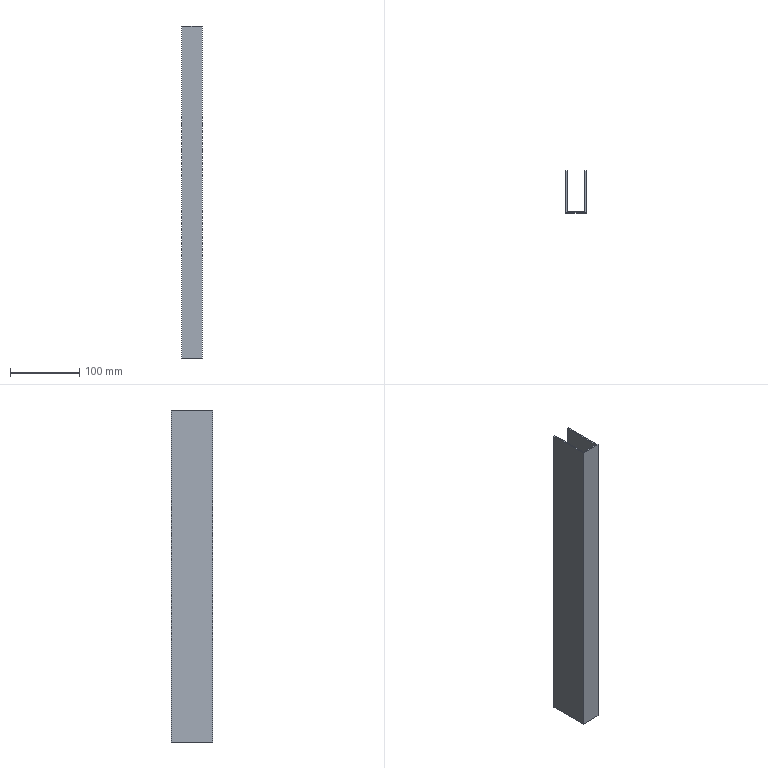Part | SolidWorks | features Extrusion 1, Shell 1 | 1 solid | 10 faces | box 30 x 60 x 480 mm | volume 140160 mm3 | plane 10
STEP:
#1=CARTESIAN_POINT('',(13.,30.,240.));
#2=VERTEX_POINT('',#1);
#3=CARTESIAN_POINT('',(13.,30.,-240.));
#4=VERTEX_POINT('',#3);
#5=CARTESIAN_POINT('',(13.,30.,240.));
#6=DIRECTION('',(0.,0.,-1.));
#7=VECTOR('',#6,1000.);
#8=LINE('',#5,#7);
#9=EDGE_CURVE('',#2,#4,#8,.T.);
#10=ORIENTED_EDGE('',*,*,#9,.F.);
#11=CARTESIAN_POINT('',(15.,30.,240.));
#12=VERTEX_POINT('',#11);
#13=CARTESIAN_POINT('',(-15.,30.,240.));
#14=DIRECTION('',(-1.,0.,0.));
#15=VECTOR('',#14,1000.);
#16=LINE('',#13,#15);
#17=EDGE_CURVE('',#12,#2,#16,.T.);
#18=ORIENTED_EDGE('',*,*,#17,.F.);
#19=CARTESIAN_POINT('',(15.,30.,-240.));
#20=VERTEX_POINT('',#19);
#21=CARTESIAN_POINT('',(15.,30.,240.));
#22=DIRECTION('',(0.,0.,-1.));
#23=VECTOR('',#22,1000.);
#24=LINE('',#21,#23);
#25=EDGE_CURVE('',#12,#20,#24,.T.);
#26=ORIENTED_EDGE('',*,*,#25,.T.);
#27=CARTESIAN_POINT('',(-15.,30.,-240.));
#28=DIRECTION('',(-1.,0.,0.));
#29=VECTOR('',#28,1000.);
#30=LINE('',#27,#29);
#31=EDGE_CURVE('',#20,#4,#30,.T.);
#32=ORIENTED_EDGE('',*,*,#31,.T.);
#33=EDGE_LOOP('',(#10,#18,#26,#32));
#34=FACE_OUTER_BOUND('',#33,.T.);
#35=CARTESIAN_POINT('',(-15.,30.,240.));
#36=DIRECTION('',(0.,-1.,0.));
#37=DIRECTION('',(0.,0.,-1.));
#38=AXIS2_PLACEMENT_3D('',#35,#36,#37);
#39=PLANE('',#38);
#40=ADVANCED_FACE('',(#34),#39,.F.);
#41=CARTESIAN_POINT('',(13.,-28.,240.));
#42=VERTEX_POINT('',#41);
#43=CARTESIAN_POINT('',(13.,0.,240.));
#44=DIRECTION('',(0.,1.,0.));
#45=VECTOR('',#44,1000.);
#46=LINE('',#43,#45);
#47=EDGE_CURVE('',#42,#2,#46,.T.);
#48=ORIENTED_EDGE('',*,*,#47,.F.);
#49=CARTESIAN_POINT('',(-13.,-28.,240.));
#50=VERTEX_POINT('',#49);
#51=CARTESIAN_POINT('',(0.,-28.,240.));
#52=DIRECTION('',(1.,0.,0.));
#53=VECTOR('',#52,1000.);
#54=LINE('',#51,#53);
#55=EDGE_CURVE('',#50,#42,#54,.T.);
#56=ORIENTED_EDGE('',*,*,#55,.F.);
#57=CARTESIAN_POINT('',(-13.,30.,240.));
#58=VERTEX_POINT('',#57);
#59=CARTESIAN_POINT('',(-13.,0.,240.));
#60=DIRECTION('',(0.,-1.,0.));
#61=VECTOR('',#60,1000.);
#62=LINE('',#59,#61);
#63=EDGE_CURVE('',#58,#50,#62,.T.);
#64=ORIENTED_EDGE('',*,*,#63,.F.);
#65=CARTESIAN_POINT('',(-15.,30.,240.));
#66=VERTEX_POINT('',#65);
#67=CARTESIAN_POINT('',(-15.,30.,240.));
#68=DIRECTION('',(-1.,0.,0.));
#69=VECTOR('',#68,1000.);
#70=LINE('',#67,#69);
#71=EDGE_CURVE('',#58,#66,#70,.T.);
#72=ORIENTED_EDGE('',*,*,#71,.T.);
#73=CARTESIAN_POINT('',(-15.,-30.,240.));
#74=VERTEX_POINT('',#73);
#75=CARTESIAN_POINT('',(-15.,-30.,240.));
#76=DIRECTION('',(0.,-1.,0.));
#77=VECTOR('',#76,1000.);
#78=LINE('',#75,#77);
#79=EDGE_CURVE('',#66,#74,#78,.T.);
#80=ORIENTED_EDGE('',*,*,#79,.T.);
#81=CARTESIAN_POINT('',(15.,-30.,240.));
#82=VERTEX_POINT('',#81);
#83=CARTESIAN_POINT('',(-15.,-30.,240.));
#84=DIRECTION('',(1.,0.,0.));
#85=VECTOR('',#84,1000.);
#86=LINE('',#83,#85);
#87=EDGE_CURVE('',#74,#82,#86,.T.);
#88=ORIENTED_EDGE('',*,*,#87,.T.);
#89=CARTESIAN_POINT('',(15.,-30.,240.));
#90=DIRECTION('',(0.,1.,0.));
#91=VECTOR('',#90,1000.);
#92=LINE('',#89,#91);
#93=EDGE_CURVE('',#82,#12,#92,.T.);
#94=ORIENTED_EDGE('',*,*,#93,.T.);
#95=ORIENTED_EDGE('',*,*,#17,.T.);
#96=EDGE_LOOP('',(#48,#56,#64,#72,#80,#88,#94,#95));
#97=FACE_OUTER_BOUND('',#96,.T.);
#98=CARTESIAN_POINT('',(0.,0.,240.));
#99=DIRECTION('',(0.,0.,-1.));
#100=DIRECTION('',(-1.,0.,0.));
#101=AXIS2_PLACEMENT_3D('',#98,#99,#100);
#102=PLANE('',#101);
#103=ADVANCED_FACE('',(#97),#102,.F.);
#104=CARTESIAN_POINT('',(-13.,-28.,-240.));
#105=VERTEX_POINT('',#104);
#106=CARTESIAN_POINT('',(13.,-28.,-240.));
#107=VERTEX_POINT('',#106);
#108=CARTESIAN_POINT('',(0.,-28.,-240.));
#109=DIRECTION('',(1.,0.,0.));
#110=VECTOR('',#109,1000.);
#111=LINE('',#108,#110);
#112=EDGE_CURVE('',#105,#107,#111,.T.);
#113=ORIENTED_EDGE('',*,*,#112,.T.);
#114=CARTESIAN_POINT('',(13.,0.,-240.));
#115=DIRECTION('',(0.,1.,0.));
#116=VECTOR('',#115,1000.);
#117=LINE('',#114,#116);
#118=EDGE_CURVE('',#107,#4,#117,.T.);
#119=ORIENTED_EDGE('',*,*,#118,.T.);
#120=ORIENTED_EDGE('',*,*,#31,.F.);
#121=CARTESIAN_POINT('',(15.,-30.,-240.));
#122=VERTEX_POINT('',#121);
#123=CARTESIAN_POINT('',(15.,-30.,-240.));
#124=DIRECTION('',(0.,1.,0.));
#125=VECTOR('',#124,1000.);
#126=LINE('',#123,#125);
#127=EDGE_CURVE('',#122,#20,#126,.T.);
#128=ORIENTED_EDGE('',*,*,#127,.F.);
#129=CARTESIAN_POINT('',(-15.,-30.,-240.));
#130=VERTEX_POINT('',#129);
#131=CARTESIAN_POINT('',(-15.,-30.,-240.));
#132=DIRECTION('',(1.,0.,0.));
#133=VECTOR('',#132,1000.);
#134=LINE('',#131,#133);
#135=EDGE_CURVE('',#130,#122,#134,.T.);
#136=ORIENTED_EDGE('',*,*,#135,.F.);
#137=CARTESIAN_POINT('',(-15.,30.,-240.));
#138=VERTEX_POINT('',#137);
#139=CARTESIAN_POINT('',(-15.,-30.,-240.));
#140=DIRECTION('',(0.,-1.,0.));
#141=VECTOR('',#140,1000.);
#142=LINE('',#139,#141);
#143=EDGE_CURVE('',#138,#130,#142,.T.);
#144=ORIENTED_EDGE('',*,*,#143,.F.);
#145=CARTESIAN_POINT('',(-13.,30.,-240.));
#146=VERTEX_POINT('',#145);
#147=CARTESIAN_POINT('',(-15.,30.,-240.));
#148=DIRECTION('',(-1.,0.,0.));
#149=VECTOR('',#148,1000.);
#150=LINE('',#147,#149);
#151=EDGE_CURVE('',#146,#138,#150,.T.);
#152=ORIENTED_EDGE('',*,*,#151,.F.);
#153=CARTESIAN_POINT('',(-13.,0.,-240.));
#154=DIRECTION('',(0.,-1.,0.));
#155=VECTOR('',#154,1000.);
#156=LINE('',#153,#155);
#157=EDGE_CURVE('',#146,#105,#156,.T.);
#158=ORIENTED_EDGE('',*,*,#157,.T.);
#159=EDGE_LOOP('',(#113,#119,#120,#128,#136,#144,#152,#158));
#160=FACE_OUTER_BOUND('',#159,.T.);
#161=CARTESIAN_POINT('',(0.,0.,-240.));
#162=DIRECTION('',(0.,0.,-1.));
#163=DIRECTION('',(-1.,0.,0.));
#164=AXIS2_PLACEMENT_3D('',#161,#162,#163);
#165=PLANE('',#164);
#166=ADVANCED_FACE('',(#160),#165,.T.);
#167=ORIENTED_EDGE('',*,*,#127,.T.);
#168=ORIENTED_EDGE('',*,*,#25,.F.);
#169=ORIENTED_EDGE('',*,*,#93,.F.);
#170=CARTESIAN_POINT('',(15.,-30.,240.));
#171=DIRECTION('',(0.,0.,-1.));
#172=VECTOR('',#171,1000.);
#173=LINE('',#170,#172);
#174=EDGE_CURVE('',#82,#122,#173,.T.);
#175=ORIENTED_EDGE('',*,*,#174,.T.);
#176=EDGE_LOOP('',(#167,#168,#169,#175));
#177=FACE_OUTER_BOUND('',#176,.T.);
#178=CARTESIAN_POINT('',(15.,-30.,240.));
#179=DIRECTION('',(-1.,0.,0.));
#180=DIRECTION('',(0.,0.,1.));
#181=AXIS2_PLACEMENT_3D('',#178,#179,#180);
#182=PLANE('',#181);
#183=ADVANCED_FACE('',(#177),#182,.F.);
#184=ORIENTED_EDGE('',*,*,#71,.F.);
#185=CARTESIAN_POINT('',(-13.,30.,240.));
#186=DIRECTION('',(0.,0.,-1.));
#187=VECTOR('',#186,1000.);
#188=LINE('',#185,#187);
#189=EDGE_CURVE('',#58,#146,#188,.T.);
#190=ORIENTED_EDGE('',*,*,#189,.T.);
#191=ORIENTED_EDGE('',*,*,#151,.T.);
#192=CARTESIAN_POINT('',(-15.,30.,240.));
#193=DIRECTION('',(0.,0.,-1.));
#194=VECTOR('',#193,1000.);
#195=LINE('',#192,#194);
#196=EDGE_CURVE('',#66,#138,#195,.T.);
#197=ORIENTED_EDGE('',*,*,#196,.F.);
#198=EDGE_LOOP('',(#184,#190,#191,#197));
#199=FACE_OUTER_BOUND('',#198,.T.);
#200=CARTESIAN_POINT('',(-15.,30.,240.));
#201=DIRECTION('',(0.,-1.,0.));
#202=DIRECTION('',(0.,0.,-1.));
#203=AXIS2_PLACEMENT_3D('',#200,#201,#202);
#204=PLANE('',#203);
#205=ADVANCED_FACE('',(#199),#204,.F.);
#206=ORIENTED_EDGE('',*,*,#143,.T.);
#207=CARTESIAN_POINT('',(-15.,-30.,240.));
#208=DIRECTION('',(0.,0.,-1.));
#209=VECTOR('',#208,1000.);
#210=LINE('',#207,#209);
#211=EDGE_CURVE('',#74,#130,#210,.T.);
#212=ORIENTED_EDGE('',*,*,#211,.F.);
#213=ORIENTED_EDGE('',*,*,#79,.F.);
#214=ORIENTED_EDGE('',*,*,#196,.T.);
#215=EDGE_LOOP('',(#206,#212,#213,#214));
#216=FACE_OUTER_BOUND('',#215,.T.);
#217=CARTESIAN_POINT('',(-15.,-30.,240.));
#218=DIRECTION('',(1.,0.,0.));
#219=DIRECTION('',(0.,0.,-1.));
#220=AXIS2_PLACEMENT_3D('',#217,#218,#219);
#221=PLANE('',#220);
#222=ADVANCED_FACE('',(#216),#221,.F.);
#223=ORIENTED_EDGE('',*,*,#135,.T.);
#224=ORIENTED_EDGE('',*,*,#174,.F.);
#225=ORIENTED_EDGE('',*,*,#87,.F.);
#226=ORIENTED_EDGE('',*,*,#211,.T.);
#227=EDGE_LOOP('',(#223,#224,#225,#226));
#228=FACE_OUTER_BOUND('',#227,.T.);
#229=CARTESIAN_POINT('',(-15.,-30.,240.));
#230=DIRECTION('',(0.,1.,0.));
#231=DIRECTION('',(0.,0.,1.));
#232=AXIS2_PLACEMENT_3D('',#229,#230,#231);
#233=PLANE('',#232);
#234=ADVANCED_FACE('',(#228),#233,.F.);
#235=ORIENTED_EDGE('',*,*,#118,.F.);
#236=CARTESIAN_POINT('',(13.,-28.,240.));
#237=DIRECTION('',(0.,0.,-1.));
#238=VECTOR('',#237,1000.);
#239=LINE('',#236,#238);
#240=EDGE_CURVE('',#42,#107,#239,.T.);
#241=ORIENTED_EDGE('',*,*,#240,.F.);
#242=ORIENTED_EDGE('',*,*,#47,.T.);
#243=ORIENTED_EDGE('',*,*,#9,.T.);
#244=EDGE_LOOP('',(#235,#241,#242,#243));
#245=FACE_OUTER_BOUND('',#244,.T.);
#246=CARTESIAN_POINT('',(13.,-30.,240.));
#247=DIRECTION('',(-1.,0.,0.));
#248=DIRECTION('',(0.,0.,1.));
#249=AXIS2_PLACEMENT_3D('',#246,#247,#248);
#250=PLANE('',#249);
#251=ADVANCED_FACE('',(#245),#250,.T.);
#252=ORIENTED_EDGE('',*,*,#157,.F.);
#253=ORIENTED_EDGE('',*,*,#189,.F.);
#254=ORIENTED_EDGE('',*,*,#63,.T.);
#255=CARTESIAN_POINT('',(-13.,-28.,240.));
#256=DIRECTION('',(0.,0.,-1.));
#257=VECTOR('',#256,1000.);
#258=LINE('',#255,#257);
#259=EDGE_CURVE('',#50,#105,#258,.T.);
#260=ORIENTED_EDGE('',*,*,#259,.T.);
#261=EDGE_LOOP('',(#252,#253,#254,#260));
#262=FACE_OUTER_BOUND('',#261,.T.);
#263=CARTESIAN_POINT('',(-13.,-30.,240.));
#264=DIRECTION('',(1.,0.,0.));
#265=DIRECTION('',(0.,0.,-1.));
#266=AXIS2_PLACEMENT_3D('',#263,#264,#265);
#267=PLANE('',#266);
#268=ADVANCED_FACE('',(#262),#267,.T.);
#269=ORIENTED_EDGE('',*,*,#112,.F.);
#270=ORIENTED_EDGE('',*,*,#259,.F.);
#271=ORIENTED_EDGE('',*,*,#55,.T.);
#272=ORIENTED_EDGE('',*,*,#240,.T.);
#273=EDGE_LOOP('',(#269,#270,#271,#272));
#274=FACE_OUTER_BOUND('',#273,.T.);
#275=CARTESIAN_POINT('',(-15.,-28.,240.));
#276=DIRECTION('',(0.,1.,0.));
#277=DIRECTION('',(0.,0.,1.));
#278=AXIS2_PLACEMENT_3D('',#275,#276,#277);
#279=PLANE('',#278);
#280=ADVANCED_FACE('',(#274),#279,.T.);
#281=CLOSED_SHELL('',(#40,#103,#166,#183,#205,#222,#234,#251,#268,#280));
#282=MANIFOLD_SOLID_BREP('',#281);
#283=CARTESIAN_POINT('',(0.,0.,0.));
#284=DIRECTION('',(0.,0.,1.));
#285=DIRECTION('',(1.,0.,0.));
#286=AXIS2_PLACEMENT_3D('',#283,#284,#285);
#287=(LENGTH_UNIT()NAMED_UNIT(*)SI_UNIT(.MILLI.,.METRE.));
#288=UNCERTAINTY_MEASURE_WITH_UNIT(LENGTH_MEASURE(0.00001),#287,'','');
#289=(NAMED_UNIT(*)PLANE_ANGLE_UNIT()SI_UNIT($,.RADIAN.));
#290=(NAMED_UNIT(*)SI_UNIT($,.STERADIAN.)SOLID_ANGLE_UNIT());
#291=(GEOMETRIC_REPRESENTATION_CONTEXT(3)GLOBAL_UNCERTAINTY_ASSIGNED_CONTEXT((#288))GLOBAL_UNIT_ASSIGNED_CONTEXT((#287,#289,#290))REPRESENTATION_CONTEXT('',''));
#292=ADVANCED_BREP_SHAPE_REPRESENTATION('',(#282,#286),#291);